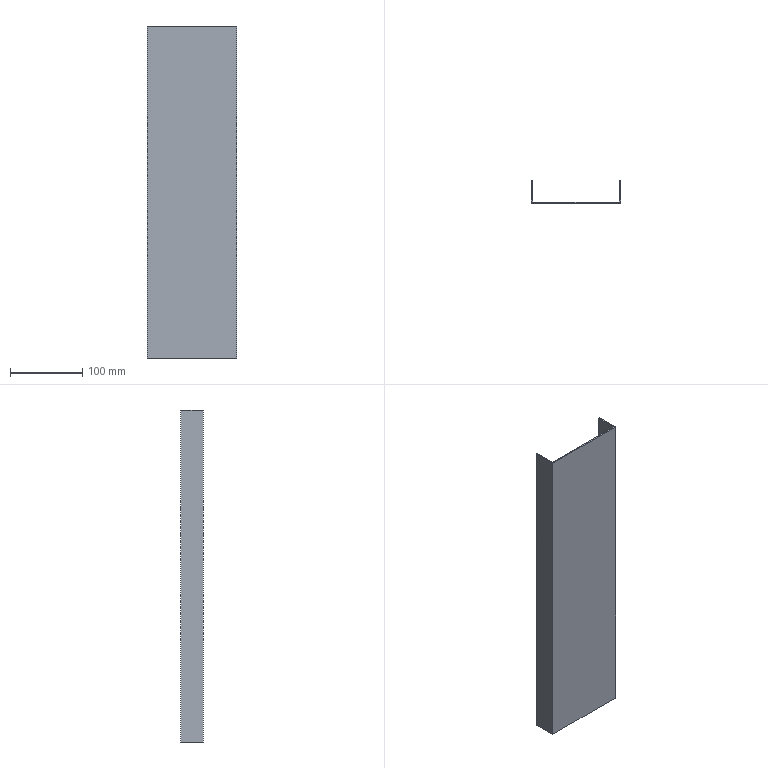Part | STEP file | Guide wheel mechanism revised.sldasm-Part-187 | 1 solid | 10 faces | box 123 x 31.5 x 458.8 mm | volume 125941 mm3 | plane 10
STEP:
#1=CARTESIAN_POINT('',(-226.,207.5,200.));
#2=VERTEX_POINT('',#1);
#3=CARTESIAN_POINT('',(-226.,239.,200.));
#4=VERTEX_POINT('',#3);
#5=CARTESIAN_POINT('',(-226.,209.,200.));
#6=DIRECTION('',(0.,1.,0.));
#7=VECTOR('',#6,1000.);
#8=LINE('',#5,#7);
#9=EDGE_CURVE('',#2,#4,#8,.T.);
#10=ORIENTED_EDGE('',*,*,#9,.T.);
#11=CARTESIAN_POINT('',(-227.5,239.,200.));
#12=VERTEX_POINT('',#11);
#13=CARTESIAN_POINT('',(-227.5,239.,200.));
#14=DIRECTION('',(1.,0.,0.));
#15=VECTOR('',#14,1000.);
#16=LINE('',#13,#15);
#17=EDGE_CURVE('',#12,#4,#16,.T.);
#18=ORIENTED_EDGE('',*,*,#17,.F.);
#19=CARTESIAN_POINT('',(-227.5,209.,200.));
#20=VERTEX_POINT('',#19);
#21=CARTESIAN_POINT('',(-227.5,209.,200.));
#22=DIRECTION('',(0.,1.,0.));
#23=VECTOR('',#22,1000.);
#24=LINE('',#21,#23);
#25=EDGE_CURVE('',#20,#12,#24,.T.);
#26=ORIENTED_EDGE('',*,*,#25,.F.);
#27=CARTESIAN_POINT('',(-347.5,209.,200.));
#28=VERTEX_POINT('',#27);
#29=CARTESIAN_POINT('',(-347.5,209.,200.));
#30=DIRECTION('',(1.,0.,0.));
#31=VECTOR('',#30,1000.);
#32=LINE('',#29,#31);
#33=EDGE_CURVE('',#28,#20,#32,.T.);
#34=ORIENTED_EDGE('',*,*,#33,.F.);
#35=CARTESIAN_POINT('',(-347.5,239.,200.));
#36=VERTEX_POINT('',#35);
#37=CARTESIAN_POINT('',(-347.5,209.,200.));
#38=DIRECTION('',(0.,-1.,0.));
#39=VECTOR('',#38,1000.);
#40=LINE('',#37,#39);
#41=EDGE_CURVE('',#36,#28,#40,.T.);
#42=ORIENTED_EDGE('',*,*,#41,.F.);
#43=CARTESIAN_POINT('',(-349.,239.,200.));
#44=VERTEX_POINT('',#43);
#45=CARTESIAN_POINT('',(-349.,239.,200.));
#46=DIRECTION('',(1.,0.,0.));
#47=VECTOR('',#46,1000.);
#48=LINE('',#45,#47);
#49=EDGE_CURVE('',#44,#36,#48,.T.);
#50=ORIENTED_EDGE('',*,*,#49,.F.);
#51=CARTESIAN_POINT('',(-349.,207.5,200.));
#52=VERTEX_POINT('',#51);
#53=CARTESIAN_POINT('',(-349.,209.,200.));
#54=DIRECTION('',(0.,-1.,0.));
#55=VECTOR('',#54,1000.);
#56=LINE('',#53,#55);
#57=EDGE_CURVE('',#44,#52,#56,.T.);
#58=ORIENTED_EDGE('',*,*,#57,.T.);
#59=CARTESIAN_POINT('',(-347.5,207.5,200.));
#60=DIRECTION('',(1.,0.,0.));
#61=VECTOR('',#60,1000.);
#62=LINE('',#59,#61);
#63=EDGE_CURVE('',#52,#2,#62,.T.);
#64=ORIENTED_EDGE('',*,*,#63,.T.);
#65=EDGE_LOOP('',(#10,#18,#26,#34,#42,#50,#58,#64));
#66=FACE_OUTER_BOUND('',#65,.T.);
#67=CARTESIAN_POINT('',(0.,0.,200.));
#68=DIRECTION('',(0.,0.,-1.));
#69=DIRECTION('',(-1.,0.,0.));
#70=AXIS2_PLACEMENT_3D('',#67,#68,#69);
#71=PLANE('',#70);
#72=ADVANCED_FACE('',(#66),#71,.F.);
#73=CARTESIAN_POINT('',(-226.,239.,-258.8));
#74=VERTEX_POINT('',#73);
#75=CARTESIAN_POINT('',(-226.,239.,-385.769));
#76=DIRECTION('',(0.,0.,1.));
#77=VECTOR('',#76,1000.);
#78=LINE('',#75,#77);
#79=EDGE_CURVE('',#74,#4,#78,.T.);
#80=ORIENTED_EDGE('',*,*,#79,.F.);
#81=CARTESIAN_POINT('',(-227.5,239.,-258.8));
#82=VERTEX_POINT('',#81);
#83=CARTESIAN_POINT('',(-227.5,239.,-258.8));
#84=DIRECTION('',(-1.,0.,0.));
#85=VECTOR('',#84,1000.);
#86=LINE('',#83,#85);
#87=EDGE_CURVE('',#74,#82,#86,.T.);
#88=ORIENTED_EDGE('',*,*,#87,.T.);
#89=CARTESIAN_POINT('',(-227.5,239.,-385.769));
#90=DIRECTION('',(0.,0.,1.));
#91=VECTOR('',#90,1000.);
#92=LINE('',#89,#91);
#93=EDGE_CURVE('',#82,#12,#92,.T.);
#94=ORIENTED_EDGE('',*,*,#93,.T.);
#95=ORIENTED_EDGE('',*,*,#17,.T.);
#96=EDGE_LOOP('',(#80,#88,#94,#95));
#97=FACE_OUTER_BOUND('',#96,.T.);
#98=CARTESIAN_POINT('',(-227.5,239.,-385.769));
#99=DIRECTION('',(0.,-1.,0.));
#100=DIRECTION('',(0.,0.,-1.));
#101=AXIS2_PLACEMENT_3D('',#98,#99,#100);
#102=PLANE('',#101);
#103=ADVANCED_FACE('',(#97),#102,.F.);
#104=ORIENTED_EDGE('',*,*,#93,.F.);
#105=CARTESIAN_POINT('',(-227.5,209.,-258.8));
#106=VERTEX_POINT('',#105);
#107=CARTESIAN_POINT('',(-227.5,209.,-258.8));
#108=DIRECTION('',(0.,-1.,0.));
#109=VECTOR('',#108,1000.);
#110=LINE('',#107,#109);
#111=EDGE_CURVE('',#82,#106,#110,.T.);
#112=ORIENTED_EDGE('',*,*,#111,.T.);
#113=CARTESIAN_POINT('',(-227.5,209.,-385.769));
#114=DIRECTION('',(0.,0.,1.));
#115=VECTOR('',#114,1000.);
#116=LINE('',#113,#115);
#117=EDGE_CURVE('',#106,#20,#116,.T.);
#118=ORIENTED_EDGE('',*,*,#117,.T.);
#119=ORIENTED_EDGE('',*,*,#25,.T.);
#120=EDGE_LOOP('',(#104,#112,#118,#119));
#121=FACE_OUTER_BOUND('',#120,.T.);
#122=CARTESIAN_POINT('',(-227.5,209.,-385.769));
#123=DIRECTION('',(1.,0.,0.));
#124=DIRECTION('',(0.,1.,0.));
#125=AXIS2_PLACEMENT_3D('',#122,#123,#124);
#126=PLANE('',#125);
#127=ADVANCED_FACE('',(#121),#126,.F.);
#128=ORIENTED_EDGE('',*,*,#117,.F.);
#129=CARTESIAN_POINT('',(-347.5,209.,-258.8));
#130=VERTEX_POINT('',#129);
#131=CARTESIAN_POINT('',(-347.5,209.,-258.8));
#132=DIRECTION('',(-1.,0.,0.));
#133=VECTOR('',#132,1000.);
#134=LINE('',#131,#133);
#135=EDGE_CURVE('',#106,#130,#134,.T.);
#136=ORIENTED_EDGE('',*,*,#135,.T.);
#137=CARTESIAN_POINT('',(-347.5,209.,-385.769));
#138=DIRECTION('',(0.,0.,1.));
#139=VECTOR('',#138,1000.);
#140=LINE('',#137,#139);
#141=EDGE_CURVE('',#130,#28,#140,.T.);
#142=ORIENTED_EDGE('',*,*,#141,.T.);
#143=ORIENTED_EDGE('',*,*,#33,.T.);
#144=EDGE_LOOP('',(#128,#136,#142,#143));
#145=FACE_OUTER_BOUND('',#144,.T.);
#146=CARTESIAN_POINT('',(-347.5,209.,-385.769));
#147=DIRECTION('',(0.,-1.,0.));
#148=DIRECTION('',(1.,0.,0.));
#149=AXIS2_PLACEMENT_3D('',#146,#147,#148);
#150=PLANE('',#149);
#151=ADVANCED_FACE('',(#145),#150,.F.);
#152=ORIENTED_EDGE('',*,*,#141,.F.);
#153=CARTESIAN_POINT('',(-347.5,239.,-258.8));
#154=VERTEX_POINT('',#153);
#155=CARTESIAN_POINT('',(-347.5,209.,-258.8));
#156=DIRECTION('',(0.,1.,0.));
#157=VECTOR('',#156,1000.);
#158=LINE('',#155,#157);
#159=EDGE_CURVE('',#130,#154,#158,.T.);
#160=ORIENTED_EDGE('',*,*,#159,.T.);
#161=CARTESIAN_POINT('',(-347.5,239.,-385.769));
#162=DIRECTION('',(0.,0.,1.));
#163=VECTOR('',#162,1000.);
#164=LINE('',#161,#163);
#165=EDGE_CURVE('',#154,#36,#164,.T.);
#166=ORIENTED_EDGE('',*,*,#165,.T.);
#167=ORIENTED_EDGE('',*,*,#41,.T.);
#168=EDGE_LOOP('',(#152,#160,#166,#167));
#169=FACE_OUTER_BOUND('',#168,.T.);
#170=CARTESIAN_POINT('',(-347.5,209.,-385.769));
#171=DIRECTION('',(-1.,0.,0.));
#172=DIRECTION('',(0.,-1.,0.));
#173=AXIS2_PLACEMENT_3D('',#170,#171,#172);
#174=PLANE('',#173);
#175=ADVANCED_FACE('',(#169),#174,.F.);
#176=ORIENTED_EDGE('',*,*,#165,.F.);
#177=CARTESIAN_POINT('',(-349.,239.,-258.8));
#178=VERTEX_POINT('',#177);
#179=CARTESIAN_POINT('',(-349.,239.,-258.8));
#180=DIRECTION('',(-1.,0.,0.));
#181=VECTOR('',#180,1000.);
#182=LINE('',#179,#181);
#183=EDGE_CURVE('',#154,#178,#182,.T.);
#184=ORIENTED_EDGE('',*,*,#183,.T.);
#185=CARTESIAN_POINT('',(-349.,239.,-385.769));
#186=DIRECTION('',(0.,0.,1.));
#187=VECTOR('',#186,1000.);
#188=LINE('',#185,#187);
#189=EDGE_CURVE('',#178,#44,#188,.T.);
#190=ORIENTED_EDGE('',*,*,#189,.T.);
#191=ORIENTED_EDGE('',*,*,#49,.T.);
#192=EDGE_LOOP('',(#176,#184,#190,#191));
#193=FACE_OUTER_BOUND('',#192,.T.);
#194=CARTESIAN_POINT('',(-349.,239.,-385.769));
#195=DIRECTION('',(0.,-1.,0.));
#196=DIRECTION('',(0.,0.,-1.));
#197=AXIS2_PLACEMENT_3D('',#194,#195,#196);
#198=PLANE('',#197);
#199=ADVANCED_FACE('',(#193),#198,.F.);
#200=CARTESIAN_POINT('',(-349.,207.5,-258.8));
#201=VERTEX_POINT('',#200);
#202=CARTESIAN_POINT('',(-349.,209.,-258.8));
#203=DIRECTION('',(0.,1.,0.));
#204=VECTOR('',#203,1000.);
#205=LINE('',#202,#204);
#206=EDGE_CURVE('',#201,#178,#205,.T.);
#207=ORIENTED_EDGE('',*,*,#206,.F.);
#208=CARTESIAN_POINT('',(-349.,207.5,-385.769));
#209=DIRECTION('',(0.,0.,1.));
#210=VECTOR('',#209,1000.);
#211=LINE('',#208,#210);
#212=EDGE_CURVE('',#201,#52,#211,.T.);
#213=ORIENTED_EDGE('',*,*,#212,.T.);
#214=ORIENTED_EDGE('',*,*,#57,.F.);
#215=ORIENTED_EDGE('',*,*,#189,.F.);
#216=EDGE_LOOP('',(#207,#213,#214,#215));
#217=FACE_OUTER_BOUND('',#216,.T.);
#218=CARTESIAN_POINT('',(-349.,209.,-385.769));
#219=DIRECTION('',(-1.,0.,0.));
#220=DIRECTION('',(0.,-1.,0.));
#221=AXIS2_PLACEMENT_3D('',#218,#219,#220);
#222=PLANE('',#221);
#223=ADVANCED_FACE('',(#217),#222,.T.);
#224=CARTESIAN_POINT('',(-226.,207.5,-258.8));
#225=VERTEX_POINT('',#224);
#226=CARTESIAN_POINT('',(-347.5,207.5,-258.8));
#227=DIRECTION('',(-1.,0.,0.));
#228=VECTOR('',#227,1000.);
#229=LINE('',#226,#228);
#230=EDGE_CURVE('',#225,#201,#229,.T.);
#231=ORIENTED_EDGE('',*,*,#230,.F.);
#232=CARTESIAN_POINT('',(-226.,207.5,-385.769));
#233=DIRECTION('',(0.,0.,1.));
#234=VECTOR('',#233,1000.);
#235=LINE('',#232,#234);
#236=EDGE_CURVE('',#225,#2,#235,.T.);
#237=ORIENTED_EDGE('',*,*,#236,.T.);
#238=ORIENTED_EDGE('',*,*,#63,.F.);
#239=ORIENTED_EDGE('',*,*,#212,.F.);
#240=EDGE_LOOP('',(#231,#237,#238,#239));
#241=FACE_OUTER_BOUND('',#240,.T.);
#242=CARTESIAN_POINT('',(-347.5,207.5,-385.769));
#243=DIRECTION('',(0.,-1.,0.));
#244=DIRECTION('',(1.,0.,0.));
#245=AXIS2_PLACEMENT_3D('',#242,#243,#244);
#246=PLANE('',#245);
#247=ADVANCED_FACE('',(#241),#246,.T.);
#248=CARTESIAN_POINT('',(-226.,209.,-258.8));
#249=DIRECTION('',(0.,-1.,0.));
#250=VECTOR('',#249,1000.);
#251=LINE('',#248,#250);
#252=EDGE_CURVE('',#74,#225,#251,.T.);
#253=ORIENTED_EDGE('',*,*,#252,.F.);
#254=ORIENTED_EDGE('',*,*,#79,.T.);
#255=ORIENTED_EDGE('',*,*,#9,.F.);
#256=ORIENTED_EDGE('',*,*,#236,.F.);
#257=EDGE_LOOP('',(#253,#254,#255,#256));
#258=FACE_OUTER_BOUND('',#257,.T.);
#259=CARTESIAN_POINT('',(-226.,209.,-385.769));
#260=DIRECTION('',(1.,0.,0.));
#261=DIRECTION('',(0.,1.,0.));
#262=AXIS2_PLACEMENT_3D('',#259,#260,#261);
#263=PLANE('',#262);
#264=ADVANCED_FACE('',(#258),#263,.T.);
#265=ORIENTED_EDGE('',*,*,#252,.T.);
#266=ORIENTED_EDGE('',*,*,#230,.T.);
#267=ORIENTED_EDGE('',*,*,#206,.T.);
#268=ORIENTED_EDGE('',*,*,#183,.F.);
#269=ORIENTED_EDGE('',*,*,#159,.F.);
#270=ORIENTED_EDGE('',*,*,#135,.F.);
#271=ORIENTED_EDGE('',*,*,#111,.F.);
#272=ORIENTED_EDGE('',*,*,#87,.F.);
#273=EDGE_LOOP('',(#265,#266,#267,#268,#269,#270,#271,#272));
#274=FACE_OUTER_BOUND('',#273,.T.);
#275=CARTESIAN_POINT('',(0.,0.,-258.8));
#276=DIRECTION('',(0.,0.,1.));
#277=DIRECTION('',(1.,0.,0.));
#278=AXIS2_PLACEMENT_3D('',#275,#276,#277);
#279=PLANE('',#278);
#280=ADVANCED_FACE('',(#274),#279,.F.);
#281=CLOSED_SHELL('',(#72,#103,#127,#151,#175,#199,#223,#247,#264,#280));
#282=MANIFOLD_SOLID_BREP('',#281);
#283=CARTESIAN_POINT('',(0.,0.,0.));
#284=DIRECTION('',(0.,0.,1.));
#285=DIRECTION('',(1.,0.,0.));
#286=AXIS2_PLACEMENT_3D('',#283,#284,#285);
#287=(LENGTH_UNIT()NAMED_UNIT(*)SI_UNIT(.MILLI.,.METRE.));
#288=UNCERTAINTY_MEASURE_WITH_UNIT(LENGTH_MEASURE(0.00001),#287,'','');
#289=(NAMED_UNIT(*)PLANE_ANGLE_UNIT()SI_UNIT($,.RADIAN.));
#290=(NAMED_UNIT(*)SI_UNIT($,.STERADIAN.)SOLID_ANGLE_UNIT());
#291=(GEOMETRIC_REPRESENTATION_CONTEXT(3)GLOBAL_UNCERTAINTY_ASSIGNED_CONTEXT((#288))GLOBAL_UNIT_ASSIGNED_CONTEXT((#287,#289,#290))REPRESENTATION_CONTEXT('',''));
#292=ADVANCED_BREP_SHAPE_REPRESENTATION('',(#282,#286),#291);